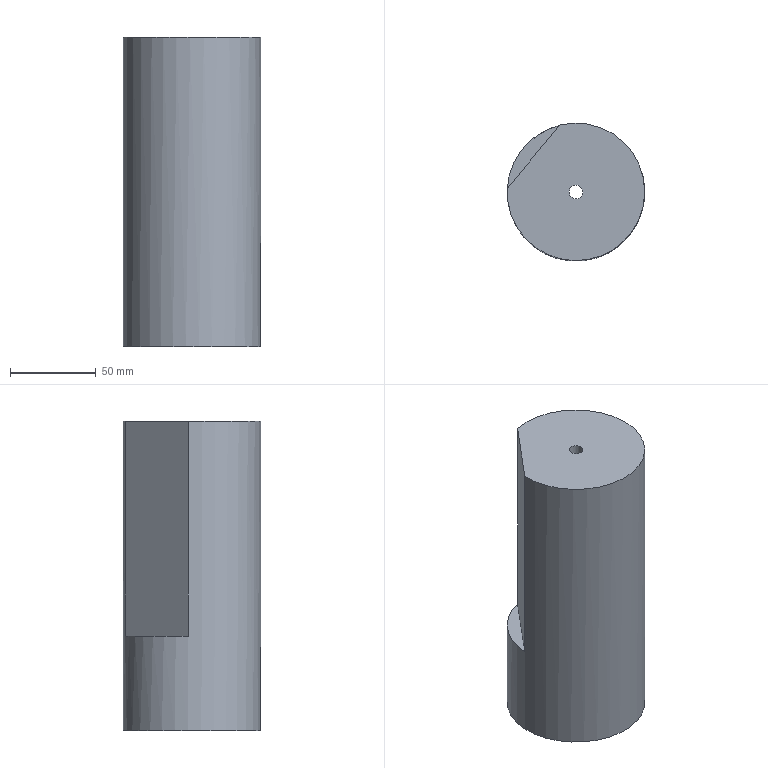Part | NX | features solid 2 | 1 solid | 8 faces | box 80 x 80 x 180 mm | volume 539643 mm3 | plane 5 | cylinder 3 | commonest cylinder face diameters 8 x1 53 x1 80 x1
STEP:
#1=CARTESIAN_POINT('',(-634.94,387.184,-30.));
#2=VERTEX_POINT('',#1);
#3=CARTESIAN_POINT('',(-634.94,387.184,-155.));
#4=VERTEX_POINT('',#3);
#5=CARTESIAN_POINT('',(-634.94,387.184,-210.));
#6=DIRECTION('',(0.,0.,1.));
#7=VECTOR('',#6,1000.);
#8=LINE('',#5,#7);
#9=EDGE_CURVE('',#2,#4,#8,.F.);
#10=ORIENTED_EDGE('',*,*,#9,.T.);
#11=CARTESIAN_POINT('',(-604.087,423.954,-155.));
#12=VERTEX_POINT('',#11);
#13=CARTESIAN_POINT('',(-595.,385.,-155.));
#14=DIRECTION('',(0.,0.,1.));
#15=DIRECTION('',(0.766,-0.6428,0.));
#16=AXIS2_PLACEMENT_3D('',#13,#14,#15);
#17=CIRCLE('',#16,40.);
#18=EDGE_CURVE('',#4,#12,#17,.F.);
#19=ORIENTED_EDGE('',*,*,#18,.T.);
#20=CARTESIAN_POINT('',(-604.087,423.954,-30.));
#21=VERTEX_POINT('',#20);
#22=CARTESIAN_POINT('',(-604.087,423.954,-210.));
#23=DIRECTION('',(0.,0.,1.));
#24=VECTOR('',#23,1000.);
#25=LINE('',#22,#24);
#26=EDGE_CURVE('',#12,#21,#25,.T.);
#27=ORIENTED_EDGE('',*,*,#26,.T.);
#28=CARTESIAN_POINT('',(-595.,385.,-30.));
#29=DIRECTION('',(0.,0.,1.));
#30=DIRECTION('',(0.766,-0.6428,0.));
#31=AXIS2_PLACEMENT_3D('',#28,#29,#30);
#32=CIRCLE('',#31,40.);
#33=EDGE_CURVE('',#21,#2,#32,.F.);
#34=ORIENTED_EDGE('',*,*,#33,.T.);
#35=EDGE_LOOP('',(#10,#19,#27,#34));
#36=FACE_BOUND('',#35,.T.);
#37=CARTESIAN_POINT('',(-564.358,359.288,-210.));
#38=VERTEX_POINT('',#37);
#39=CARTESIAN_POINT('',(-595.,385.,-210.));
#40=DIRECTION('',(0.,0.,1.));
#41=DIRECTION('',(0.766,-0.6428,0.));
#42=AXIS2_PLACEMENT_3D('',#39,#40,#41);
#43=CIRCLE('',#42,40.);
#44=EDGE_CURVE('',#38,#38,#43,.F.);
#45=ORIENTED_EDGE('',*,*,#44,.F.);
#46=EDGE_LOOP('',(#45));
#47=FACE_BOUND('',#46,.T.);
#48=CARTESIAN_POINT('',(-595.,385.,-210.));
#49=DIRECTION('',(0.,0.,1.));
#50=DIRECTION('',(-0.766,0.6428,0.));
#51=AXIS2_PLACEMENT_3D('',#48,#49,#50);
#52=CYLINDRICAL_SURFACE('',#51,40.);
#53=ADVANCED_FACE('',(#36,#47),#52,.T.);
#54=CARTESIAN_POINT('',(-615.3,402.034,-210.));
#55=VERTEX_POINT('',#54);
#56=CARTESIAN_POINT('',(-595.,385.,-210.));
#57=DIRECTION('',(0.,0.,-1.));
#58=DIRECTION('',(-0.766,0.6428,0.));
#59=AXIS2_PLACEMENT_3D('',#56,#57,#58);
#60=CIRCLE('',#59,26.5);
#61=EDGE_CURVE('',#55,#55,#60,.T.);
#62=ORIENTED_EDGE('',*,*,#61,.F.);
#63=EDGE_LOOP('',(#62));
#64=FACE_BOUND('',#63,.T.);
#65=ORIENTED_EDGE('',*,*,#44,.T.);
#66=EDGE_LOOP('',(#65));
#67=FACE_BOUND('',#66,.T.);
#68=CARTESIAN_POINT('',(-595.,385.,-210.));
#69=DIRECTION('',(0.,0.,-1.));
#70=DIRECTION('',(0.766,-0.6428,0.));
#71=AXIS2_PLACEMENT_3D('',#68,#69,#70);
#72=PLANE('',#71);
#73=ADVANCED_FACE('',(#64,#67),#72,.T.);
#74=CARTESIAN_POINT('',(-591.936,382.429,-30.));
#75=VERTEX_POINT('',#74);
#76=CARTESIAN_POINT('',(-595.,385.,-30.));
#77=DIRECTION('',(0.,0.,1.));
#78=DIRECTION('',(0.766,-0.6428,0.));
#79=AXIS2_PLACEMENT_3D('',#76,#77,#78);
#80=CIRCLE('',#79,4.);
#81=EDGE_CURVE('',#75,#75,#80,.T.);
#82=ORIENTED_EDGE('',*,*,#81,.F.);
#83=EDGE_LOOP('',(#82));
#84=FACE_BOUND('',#83,.T.);
#85=ORIENTED_EDGE('',*,*,#33,.F.);
#86=CARTESIAN_POINT('',(-593.802,436.211,-30.));
#87=DIRECTION('',(-0.6428,-0.766,0.));
#88=VECTOR('',#87,1000.);
#89=LINE('',#86,#88);
#90=EDGE_CURVE('',#21,#2,#89,.T.);
#91=ORIENTED_EDGE('',*,*,#90,.T.);
#92=EDGE_LOOP('',(#85,#91));
#93=FACE_BOUND('',#92,.T.);
#94=CARTESIAN_POINT('',(-595.,385.,-30.));
#95=DIRECTION('',(0.,0.,-1.));
#96=DIRECTION('',(0.766,-0.6428,0.));
#97=AXIS2_PLACEMENT_3D('',#94,#95,#96);
#98=PLANE('',#97);
#99=ADVANCED_FACE('',(#84,#93),#98,.F.);
#100=CARTESIAN_POINT('',(-598.064,387.571,-60.));
#101=VERTEX_POINT('',#100);
#102=CARTESIAN_POINT('',(-595.,385.,-60.));
#103=DIRECTION('',(0.,0.,-1.));
#104=DIRECTION('',(-0.766,0.6428,0.));
#105=AXIS2_PLACEMENT_3D('',#102,#103,#104);
#106=CIRCLE('',#105,4.);
#107=EDGE_CURVE('',#101,#101,#106,.T.);
#108=ORIENTED_EDGE('',*,*,#107,.F.);
#109=EDGE_LOOP('',(#108));
#110=FACE_BOUND('',#109,.T.);
#111=CARTESIAN_POINT('',(-615.3,402.034,-60.));
#112=VERTEX_POINT('',#111);
#113=CARTESIAN_POINT('',(-595.,385.,-60.));
#114=DIRECTION('',(0.,0.,-1.));
#115=DIRECTION('',(-0.766,0.6428,0.));
#116=AXIS2_PLACEMENT_3D('',#113,#114,#115);
#117=CIRCLE('',#116,26.5);
#118=EDGE_CURVE('',#112,#112,#117,.T.);
#119=ORIENTED_EDGE('',*,*,#118,.T.);
#120=EDGE_LOOP('',(#119));
#121=FACE_BOUND('',#120,.T.);
#122=CARTESIAN_POINT('',(-595.,385.,-60.));
#123=DIRECTION('',(0.,0.,1.));
#124=DIRECTION('',(-0.766,0.6428,0.));
#125=AXIS2_PLACEMENT_3D('',#122,#123,#124);
#126=PLANE('',#125);
#127=ADVANCED_FACE('',(#110,#121),#126,.F.);
#128=ORIENTED_EDGE('',*,*,#118,.F.);
#129=EDGE_LOOP('',(#128));
#130=FACE_BOUND('',#129,.T.);
#131=ORIENTED_EDGE('',*,*,#61,.T.);
#132=EDGE_LOOP('',(#131));
#133=FACE_BOUND('',#132,.T.);
#134=CARTESIAN_POINT('',(-595.,385.,-210.));
#135=DIRECTION('',(0.,0.,1.));
#136=DIRECTION('',(-0.766,0.6428,0.));
#137=AXIS2_PLACEMENT_3D('',#134,#135,#136);
#138=CYLINDRICAL_SURFACE('',#137,26.5);
#139=ADVANCED_FACE('',(#130,#133),#138,.F.);
#140=ORIENTED_EDGE('',*,*,#18,.F.);
#141=CARTESIAN_POINT('',(-593.802,436.211,-155.));
#142=DIRECTION('',(-0.6428,-0.766,0.));
#143=VECTOR('',#142,1000.);
#144=LINE('',#141,#143);
#145=EDGE_CURVE('',#12,#4,#144,.T.);
#146=ORIENTED_EDGE('',*,*,#145,.F.);
#147=EDGE_LOOP('',(#140,#146));
#148=FACE_BOUND('',#147,.T.);
#149=CARTESIAN_POINT('',(-569.288,415.642,-155.));
#150=DIRECTION('',(0.,0.,-1.));
#151=DIRECTION('',(-0.6428,-0.766,0.));
#152=AXIS2_PLACEMENT_3D('',#149,#150,#151);
#153=PLANE('',#152);
#154=ADVANCED_FACE('',(#148),#153,.F.);
#155=ORIENTED_EDGE('',*,*,#9,.F.);
#156=ORIENTED_EDGE('',*,*,#90,.F.);
#157=ORIENTED_EDGE('',*,*,#26,.F.);
#158=ORIENTED_EDGE('',*,*,#145,.T.);
#159=EDGE_LOOP('',(#155,#156,#157,#158));
#160=FACE_BOUND('',#159,.T.);
#161=CARTESIAN_POINT('',(-593.802,436.211,-155.));
#162=DIRECTION('',(0.766,-0.6428,0.));
#163=DIRECTION('',(-0.6428,-0.766,0.));
#164=AXIS2_PLACEMENT_3D('',#161,#162,#163);
#165=PLANE('',#164);
#166=ADVANCED_FACE('',(#160),#165,.F.);
#167=ORIENTED_EDGE('',*,*,#81,.T.);
#168=EDGE_LOOP('',(#167));
#169=FACE_BOUND('',#168,.T.);
#170=ORIENTED_EDGE('',*,*,#107,.T.);
#171=EDGE_LOOP('',(#170));
#172=FACE_BOUND('',#171,.T.);
#173=CARTESIAN_POINT('',(-595.,385.,-30.));
#174=DIRECTION('',(0.,0.,-1.));
#175=DIRECTION('',(0.766,-0.6428,0.));
#176=AXIS2_PLACEMENT_3D('',#173,#174,#175);
#177=CYLINDRICAL_SURFACE('',#176,4.);
#178=ADVANCED_FACE('',(#169,#172),#177,.F.);
#179=CLOSED_SHELL('',(#53,#73,#99,#127,#139,#154,#166,#178));
#180=MANIFOLD_SOLID_BREP('',#179);
#181=(LENGTH_UNIT()NAMED_UNIT(*)SI_UNIT(.MILLI.,.METRE.));
#182=UNCERTAINTY_MEASURE_WITH_UNIT(LENGTH_MEASURE(0.00001),#181,'','');
#183=(NAMED_UNIT(*)PLANE_ANGLE_UNIT()SI_UNIT($,.RADIAN.));
#184=(NAMED_UNIT(*)SI_UNIT($,.STERADIAN.)SOLID_ANGLE_UNIT());
#185=(GEOMETRIC_REPRESENTATION_CONTEXT(3)GLOBAL_UNCERTAINTY_ASSIGNED_CONTEXT((#182))GLOBAL_UNIT_ASSIGNED_CONTEXT((#181,#183,#184))REPRESENTATION_CONTEXT('',''));
#186=ADVANCED_BREP_SHAPE_REPRESENTATION('',(#180),#185);